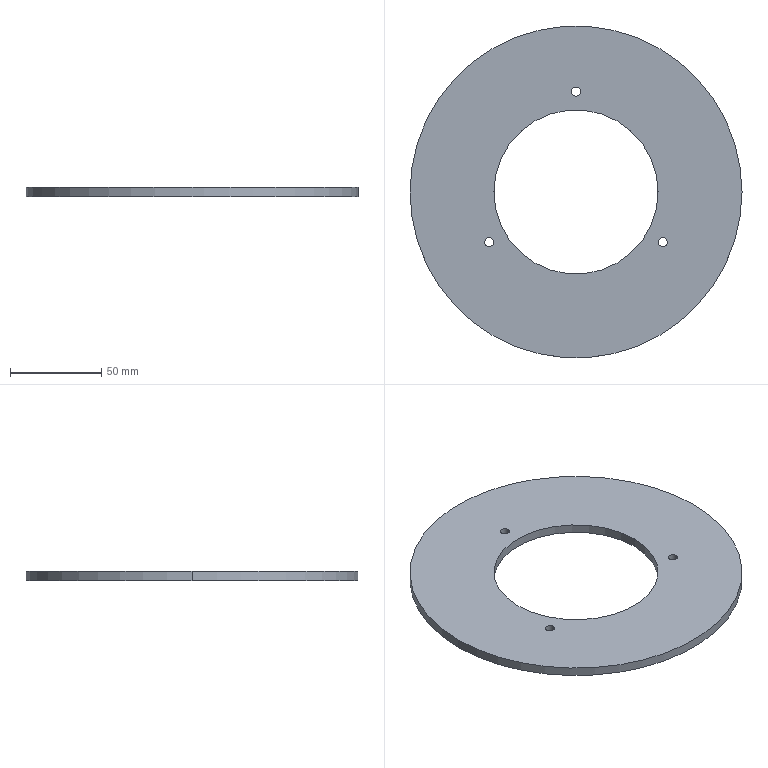Part | SolidWorks | features Extrusion 1 | 1 solid | 12 faces | box 182 x 182 x 5 mm | volume 97974 mm3 | cylinder 10 | plane 2 | commonest cylinder face diameters 5 x6 90 x2 182 x2
STEP:
#1=CARTESIAN_POINT('',(-50.131,-27.5,5.));
#2=VERTEX_POINT('',#1);
#3=CARTESIAN_POINT('',(-45.131,-27.5,5.));
#4=VERTEX_POINT('',#3);
#5=CARTESIAN_POINT('',(-47.631,-27.5,5.));
#6=DIRECTION('',(0.,0.,1.));
#7=DIRECTION('',(1.,0.,0.));
#8=AXIS2_PLACEMENT_3D('',#5,#6,#7);
#9=CIRCLE('',#8,2.5);
#10=EDGE_CURVE('',#2,#4,#9,.T.);
#11=ORIENTED_EDGE('',*,*,#10,.T.);
#12=CARTESIAN_POINT('',(-45.131,-27.5,0.));
#13=VERTEX_POINT('',#12);
#14=CARTESIAN_POINT('',(-45.131,-27.5,5.));
#15=DIRECTION('',(0.,0.,-1.));
#16=VECTOR('',#15,1000.);
#17=LINE('',#14,#16);
#18=EDGE_CURVE('',#4,#13,#17,.T.);
#19=ORIENTED_EDGE('',*,*,#18,.T.);
#20=CARTESIAN_POINT('',(-50.131,-27.5,0.));
#21=VERTEX_POINT('',#20);
#22=CARTESIAN_POINT('',(-47.631,-27.5,0.));
#23=DIRECTION('',(0.,0.,1.));
#24=DIRECTION('',(1.,0.,0.));
#25=AXIS2_PLACEMENT_3D('',#22,#23,#24);
#26=CIRCLE('',#25,2.5);
#27=EDGE_CURVE('',#21,#13,#26,.T.);
#28=ORIENTED_EDGE('',*,*,#27,.F.);
#29=CARTESIAN_POINT('',(-50.131,-27.5,5.));
#30=DIRECTION('',(0.,0.,-1.));
#31=VECTOR('',#30,1000.);
#32=LINE('',#29,#31);
#33=EDGE_CURVE('',#2,#21,#32,.T.);
#34=ORIENTED_EDGE('',*,*,#33,.F.);
#35=EDGE_LOOP('',(#11,#19,#28,#34));
#36=FACE_OUTER_BOUND('',#35,.T.);
#37=CARTESIAN_POINT('',(-47.631,-27.5,5.));
#38=DIRECTION('',(0.,0.,-1.));
#39=DIRECTION('',(-1.,0.,0.));
#40=AXIS2_PLACEMENT_3D('',#37,#38,#39);
#41=CYLINDRICAL_SURFACE('',#40,2.5);
#42=ADVANCED_FACE('',(#36),#41,.F.);
#43=CARTESIAN_POINT('',(45.131,-27.5,5.));
#44=VERTEX_POINT('',#43);
#45=CARTESIAN_POINT('',(50.131,-27.5,5.));
#46=VERTEX_POINT('',#45);
#47=CARTESIAN_POINT('',(47.631,-27.5,5.));
#48=DIRECTION('',(0.,0.,1.));
#49=DIRECTION('',(1.,0.,0.));
#50=AXIS2_PLACEMENT_3D('',#47,#48,#49);
#51=CIRCLE('',#50,2.5);
#52=EDGE_CURVE('',#44,#46,#51,.T.);
#53=ORIENTED_EDGE('',*,*,#52,.T.);
#54=CARTESIAN_POINT('',(50.131,-27.5,0.));
#55=VERTEX_POINT('',#54);
#56=CARTESIAN_POINT('',(50.131,-27.5,5.));
#57=DIRECTION('',(0.,0.,-1.));
#58=VECTOR('',#57,1000.);
#59=LINE('',#56,#58);
#60=EDGE_CURVE('',#46,#55,#59,.T.);
#61=ORIENTED_EDGE('',*,*,#60,.T.);
#62=CARTESIAN_POINT('',(45.131,-27.5,0.));
#63=VERTEX_POINT('',#62);
#64=CARTESIAN_POINT('',(47.631,-27.5,0.));
#65=DIRECTION('',(0.,0.,1.));
#66=DIRECTION('',(1.,0.,0.));
#67=AXIS2_PLACEMENT_3D('',#64,#65,#66);
#68=CIRCLE('',#67,2.5);
#69=EDGE_CURVE('',#63,#55,#68,.T.);
#70=ORIENTED_EDGE('',*,*,#69,.F.);
#71=CARTESIAN_POINT('',(45.131,-27.5,5.));
#72=DIRECTION('',(0.,0.,-1.));
#73=VECTOR('',#72,1000.);
#74=LINE('',#71,#73);
#75=EDGE_CURVE('',#44,#63,#74,.T.);
#76=ORIENTED_EDGE('',*,*,#75,.F.);
#77=EDGE_LOOP('',(#53,#61,#70,#76));
#78=FACE_OUTER_BOUND('',#77,.T.);
#79=CARTESIAN_POINT('',(47.631,-27.5,5.));
#80=DIRECTION('',(0.,0.,-1.));
#81=DIRECTION('',(-1.,0.,0.));
#82=AXIS2_PLACEMENT_3D('',#79,#80,#81);
#83=CYLINDRICAL_SURFACE('',#82,2.5);
#84=ADVANCED_FACE('',(#78),#83,.F.);
#85=CARTESIAN_POINT('',(-2.5,55.,5.));
#86=VERTEX_POINT('',#85);
#87=CARTESIAN_POINT('',(2.5,55.,5.));
#88=VERTEX_POINT('',#87);
#89=CARTESIAN_POINT('',(0.,55.,5.));
#90=DIRECTION('',(0.,0.,1.));
#91=DIRECTION('',(1.,0.,0.));
#92=AXIS2_PLACEMENT_3D('',#89,#90,#91);
#93=CIRCLE('',#92,2.5);
#94=EDGE_CURVE('',#86,#88,#93,.T.);
#95=ORIENTED_EDGE('',*,*,#94,.T.);
#96=CARTESIAN_POINT('',(2.5,55.,0.));
#97=VERTEX_POINT('',#96);
#98=CARTESIAN_POINT('',(2.5,55.,5.));
#99=DIRECTION('',(0.,0.,-1.));
#100=VECTOR('',#99,1000.);
#101=LINE('',#98,#100);
#102=EDGE_CURVE('',#88,#97,#101,.T.);
#103=ORIENTED_EDGE('',*,*,#102,.T.);
#104=CARTESIAN_POINT('',(-2.5,55.,0.));
#105=VERTEX_POINT('',#104);
#106=CARTESIAN_POINT('',(0.,55.,0.));
#107=DIRECTION('',(0.,0.,1.));
#108=DIRECTION('',(1.,0.,0.));
#109=AXIS2_PLACEMENT_3D('',#106,#107,#108);
#110=CIRCLE('',#109,2.5);
#111=EDGE_CURVE('',#105,#97,#110,.T.);
#112=ORIENTED_EDGE('',*,*,#111,.F.);
#113=CARTESIAN_POINT('',(-2.5,55.,5.));
#114=DIRECTION('',(0.,0.,-1.));
#115=VECTOR('',#114,1000.);
#116=LINE('',#113,#115);
#117=EDGE_CURVE('',#86,#105,#116,.T.);
#118=ORIENTED_EDGE('',*,*,#117,.F.);
#119=EDGE_LOOP('',(#95,#103,#112,#118));
#120=FACE_OUTER_BOUND('',#119,.T.);
#121=CARTESIAN_POINT('',(0.,55.,5.));
#122=DIRECTION('',(0.,0.,-1.));
#123=DIRECTION('',(-1.,0.,0.));
#124=AXIS2_PLACEMENT_3D('',#121,#122,#123);
#125=CYLINDRICAL_SURFACE('',#124,2.5);
#126=ADVANCED_FACE('',(#120),#125,.F.);
#127=CARTESIAN_POINT('',(-45.,0.,5.));
#128=VERTEX_POINT('',#127);
#129=CARTESIAN_POINT('',(45.,0.,5.));
#130=VERTEX_POINT('',#129);
#131=CARTESIAN_POINT('',(0.,0.,5.));
#132=DIRECTION('',(0.,0.,1.));
#133=DIRECTION('',(1.,0.,0.));
#134=AXIS2_PLACEMENT_3D('',#131,#132,#133);
#135=CIRCLE('',#134,45.);
#136=EDGE_CURVE('',#128,#130,#135,.T.);
#137=ORIENTED_EDGE('',*,*,#136,.T.);
#138=CARTESIAN_POINT('',(45.,0.,0.));
#139=VERTEX_POINT('',#138);
#140=CARTESIAN_POINT('',(45.,0.,5.));
#141=DIRECTION('',(0.,0.,-1.));
#142=VECTOR('',#141,1000.);
#143=LINE('',#140,#142);
#144=EDGE_CURVE('',#130,#139,#143,.T.);
#145=ORIENTED_EDGE('',*,*,#144,.T.);
#146=CARTESIAN_POINT('',(-45.,0.,0.));
#147=VERTEX_POINT('',#146);
#148=CARTESIAN_POINT('',(0.,0.,0.));
#149=DIRECTION('',(0.,0.,1.));
#150=DIRECTION('',(1.,0.,0.));
#151=AXIS2_PLACEMENT_3D('',#148,#149,#150);
#152=CIRCLE('',#151,45.);
#153=EDGE_CURVE('',#147,#139,#152,.T.);
#154=ORIENTED_EDGE('',*,*,#153,.F.);
#155=CARTESIAN_POINT('',(-45.,0.,5.));
#156=DIRECTION('',(0.,0.,-1.));
#157=VECTOR('',#156,1000.);
#158=LINE('',#155,#157);
#159=EDGE_CURVE('',#128,#147,#158,.T.);
#160=ORIENTED_EDGE('',*,*,#159,.F.);
#161=EDGE_LOOP('',(#137,#145,#154,#160));
#162=FACE_OUTER_BOUND('',#161,.T.);
#163=CARTESIAN_POINT('',(0.,0.,5.));
#164=DIRECTION('',(0.,0.,-1.));
#165=DIRECTION('',(-1.,0.,0.));
#166=AXIS2_PLACEMENT_3D('',#163,#164,#165);
#167=CYLINDRICAL_SURFACE('',#166,45.);
#168=ADVANCED_FACE('',(#162),#167,.F.);
#169=CARTESIAN_POINT('',(91.,0.,5.));
#170=VERTEX_POINT('',#169);
#171=CARTESIAN_POINT('',(-91.,0.,5.));
#172=VERTEX_POINT('',#171);
#173=CARTESIAN_POINT('',(0.,0.,5.));
#174=DIRECTION('',(0.,0.,1.));
#175=DIRECTION('',(1.,0.,0.));
#176=AXIS2_PLACEMENT_3D('',#173,#174,#175);
#177=CIRCLE('',#176,91.);
#178=EDGE_CURVE('',#170,#172,#177,.T.);
#179=ORIENTED_EDGE('',*,*,#178,.F.);
#180=CARTESIAN_POINT('',(91.,0.,0.));
#181=VERTEX_POINT('',#180);
#182=CARTESIAN_POINT('',(91.,0.,5.));
#183=DIRECTION('',(0.,0.,-1.));
#184=VECTOR('',#183,1000.);
#185=LINE('',#182,#184);
#186=EDGE_CURVE('',#170,#181,#185,.T.);
#187=ORIENTED_EDGE('',*,*,#186,.T.);
#188=CARTESIAN_POINT('',(-91.,0.,0.));
#189=VERTEX_POINT('',#188);
#190=CARTESIAN_POINT('',(0.,0.,0.));
#191=DIRECTION('',(0.,0.,1.));
#192=DIRECTION('',(1.,0.,0.));
#193=AXIS2_PLACEMENT_3D('',#190,#191,#192);
#194=CIRCLE('',#193,91.);
#195=EDGE_CURVE('',#181,#189,#194,.T.);
#196=ORIENTED_EDGE('',*,*,#195,.T.);
#197=CARTESIAN_POINT('',(-91.,0.,5.));
#198=DIRECTION('',(0.,0.,-1.));
#199=VECTOR('',#198,1000.);
#200=LINE('',#197,#199);
#201=EDGE_CURVE('',#172,#189,#200,.T.);
#202=ORIENTED_EDGE('',*,*,#201,.F.);
#203=EDGE_LOOP('',(#179,#187,#196,#202));
#204=FACE_OUTER_BOUND('',#203,.T.);
#205=CARTESIAN_POINT('',(0.,0.,5.));
#206=DIRECTION('',(0.,0.,-1.));
#207=DIRECTION('',(-1.,0.,0.));
#208=AXIS2_PLACEMENT_3D('',#205,#206,#207);
#209=CYLINDRICAL_SURFACE('',#208,91.);
#210=ADVANCED_FACE('',(#204),#209,.T.);
#211=ORIENTED_EDGE('',*,*,#52,.F.);
#212=CARTESIAN_POINT('',(47.631,-27.5,5.));
#213=DIRECTION('',(0.,0.,1.));
#214=DIRECTION('',(1.,0.,0.));
#215=AXIS2_PLACEMENT_3D('',#212,#213,#214);
#216=CIRCLE('',#215,2.5);
#217=EDGE_CURVE('',#46,#44,#216,.T.);
#218=ORIENTED_EDGE('',*,*,#217,.F.);
#219=EDGE_LOOP('',(#211,#218));
#220=FACE_BOUND('',#219,.T.);
#221=ORIENTED_EDGE('',*,*,#136,.F.);
#222=CARTESIAN_POINT('',(0.,0.,5.));
#223=DIRECTION('',(0.,0.,1.));
#224=DIRECTION('',(1.,0.,0.));
#225=AXIS2_PLACEMENT_3D('',#222,#223,#224);
#226=CIRCLE('',#225,45.);
#227=EDGE_CURVE('',#130,#128,#226,.T.);
#228=ORIENTED_EDGE('',*,*,#227,.F.);
#229=EDGE_LOOP('',(#221,#228));
#230=FACE_BOUND('',#229,.T.);
#231=CARTESIAN_POINT('',(0.,0.,5.));
#232=DIRECTION('',(0.,0.,1.));
#233=DIRECTION('',(1.,0.,0.));
#234=AXIS2_PLACEMENT_3D('',#231,#232,#233);
#235=CIRCLE('',#234,91.);
#236=EDGE_CURVE('',#172,#170,#235,.T.);
#237=ORIENTED_EDGE('',*,*,#236,.T.);
#238=ORIENTED_EDGE('',*,*,#178,.T.);
#239=EDGE_LOOP('',(#237,#238));
#240=FACE_OUTER_BOUND('',#239,.T.);
#241=ORIENTED_EDGE('',*,*,#94,.F.);
#242=CARTESIAN_POINT('',(0.,55.,5.));
#243=DIRECTION('',(0.,0.,1.));
#244=DIRECTION('',(1.,0.,0.));
#245=AXIS2_PLACEMENT_3D('',#242,#243,#244);
#246=CIRCLE('',#245,2.5);
#247=EDGE_CURVE('',#88,#86,#246,.T.);
#248=ORIENTED_EDGE('',*,*,#247,.F.);
#249=EDGE_LOOP('',(#241,#248));
#250=FACE_BOUND('',#249,.T.);
#251=ORIENTED_EDGE('',*,*,#10,.F.);
#252=CARTESIAN_POINT('',(-47.631,-27.5,5.));
#253=DIRECTION('',(0.,0.,1.));
#254=DIRECTION('',(1.,0.,0.));
#255=AXIS2_PLACEMENT_3D('',#252,#253,#254);
#256=CIRCLE('',#255,2.5);
#257=EDGE_CURVE('',#4,#2,#256,.T.);
#258=ORIENTED_EDGE('',*,*,#257,.F.);
#259=EDGE_LOOP('',(#251,#258));
#260=FACE_BOUND('',#259,.T.);
#261=CARTESIAN_POINT('',(0.,0.,5.));
#262=DIRECTION('',(0.,0.,1.));
#263=DIRECTION('',(1.,0.,0.));
#264=AXIS2_PLACEMENT_3D('',#261,#262,#263);
#265=PLANE('',#264);
#266=ADVANCED_FACE('',(#220,#230,#240,#250,#260),#265,.T.);
#267=CARTESIAN_POINT('',(0.,0.,0.));
#268=DIRECTION('',(0.,0.,1.));
#269=DIRECTION('',(1.,0.,0.));
#270=AXIS2_PLACEMENT_3D('',#267,#268,#269);
#271=CIRCLE('',#270,91.);
#272=EDGE_CURVE('',#189,#181,#271,.T.);
#273=ORIENTED_EDGE('',*,*,#272,.F.);
#274=ORIENTED_EDGE('',*,*,#195,.F.);
#275=EDGE_LOOP('',(#273,#274));
#276=FACE_OUTER_BOUND('',#275,.T.);
#277=ORIENTED_EDGE('',*,*,#153,.T.);
#278=CARTESIAN_POINT('',(0.,0.,0.));
#279=DIRECTION('',(0.,0.,1.));
#280=DIRECTION('',(1.,0.,0.));
#281=AXIS2_PLACEMENT_3D('',#278,#279,#280);
#282=CIRCLE('',#281,45.);
#283=EDGE_CURVE('',#139,#147,#282,.T.);
#284=ORIENTED_EDGE('',*,*,#283,.T.);
#285=EDGE_LOOP('',(#277,#284));
#286=FACE_BOUND('',#285,.T.);
#287=ORIENTED_EDGE('',*,*,#111,.T.);
#288=CARTESIAN_POINT('',(0.,55.,0.));
#289=DIRECTION('',(0.,0.,1.));
#290=DIRECTION('',(1.,0.,0.));
#291=AXIS2_PLACEMENT_3D('',#288,#289,#290);
#292=CIRCLE('',#291,2.5);
#293=EDGE_CURVE('',#97,#105,#292,.T.);
#294=ORIENTED_EDGE('',*,*,#293,.T.);
#295=EDGE_LOOP('',(#287,#294));
#296=FACE_BOUND('',#295,.T.);
#297=ORIENTED_EDGE('',*,*,#69,.T.);
#298=CARTESIAN_POINT('',(47.631,-27.5,0.));
#299=DIRECTION('',(0.,0.,1.));
#300=DIRECTION('',(1.,0.,0.));
#301=AXIS2_PLACEMENT_3D('',#298,#299,#300);
#302=CIRCLE('',#301,2.5);
#303=EDGE_CURVE('',#55,#63,#302,.T.);
#304=ORIENTED_EDGE('',*,*,#303,.T.);
#305=EDGE_LOOP('',(#297,#304));
#306=FACE_BOUND('',#305,.T.);
#307=ORIENTED_EDGE('',*,*,#27,.T.);
#308=CARTESIAN_POINT('',(-47.631,-27.5,0.));
#309=DIRECTION('',(0.,0.,1.));
#310=DIRECTION('',(1.,0.,0.));
#311=AXIS2_PLACEMENT_3D('',#308,#309,#310);
#312=CIRCLE('',#311,2.5);
#313=EDGE_CURVE('',#13,#21,#312,.T.);
#314=ORIENTED_EDGE('',*,*,#313,.T.);
#315=EDGE_LOOP('',(#307,#314));
#316=FACE_BOUND('',#315,.T.);
#317=CARTESIAN_POINT('',(0.,0.,0.));
#318=DIRECTION('',(0.,0.,1.));
#319=DIRECTION('',(1.,0.,0.));
#320=AXIS2_PLACEMENT_3D('',#317,#318,#319);
#321=PLANE('',#320);
#322=ADVANCED_FACE('',(#276,#286,#296,#306,#316),#321,.F.);
#323=ORIENTED_EDGE('',*,*,#186,.F.);
#324=ORIENTED_EDGE('',*,*,#236,.F.);
#325=ORIENTED_EDGE('',*,*,#201,.T.);
#326=ORIENTED_EDGE('',*,*,#272,.T.);
#327=EDGE_LOOP('',(#323,#324,#325,#326));
#328=FACE_OUTER_BOUND('',#327,.T.);
#329=CARTESIAN_POINT('',(0.,0.,5.));
#330=DIRECTION('',(0.,0.,-1.));
#331=DIRECTION('',(-1.,0.,0.));
#332=AXIS2_PLACEMENT_3D('',#329,#330,#331);
#333=CYLINDRICAL_SURFACE('',#332,91.);
#334=ADVANCED_FACE('',(#328),#333,.T.);
#335=ORIENTED_EDGE('',*,*,#144,.F.);
#336=ORIENTED_EDGE('',*,*,#227,.T.);
#337=ORIENTED_EDGE('',*,*,#159,.T.);
#338=ORIENTED_EDGE('',*,*,#283,.F.);
#339=EDGE_LOOP('',(#335,#336,#337,#338));
#340=FACE_OUTER_BOUND('',#339,.T.);
#341=CARTESIAN_POINT('',(0.,0.,5.));
#342=DIRECTION('',(0.,0.,-1.));
#343=DIRECTION('',(-1.,0.,0.));
#344=AXIS2_PLACEMENT_3D('',#341,#342,#343);
#345=CYLINDRICAL_SURFACE('',#344,45.);
#346=ADVANCED_FACE('',(#340),#345,.F.);
#347=ORIENTED_EDGE('',*,*,#102,.F.);
#348=ORIENTED_EDGE('',*,*,#247,.T.);
#349=ORIENTED_EDGE('',*,*,#117,.T.);
#350=ORIENTED_EDGE('',*,*,#293,.F.);
#351=EDGE_LOOP('',(#347,#348,#349,#350));
#352=FACE_OUTER_BOUND('',#351,.T.);
#353=CARTESIAN_POINT('',(0.,55.,5.));
#354=DIRECTION('',(0.,0.,-1.));
#355=DIRECTION('',(-1.,0.,0.));
#356=AXIS2_PLACEMENT_3D('',#353,#354,#355);
#357=CYLINDRICAL_SURFACE('',#356,2.5);
#358=ADVANCED_FACE('',(#352),#357,.F.);
#359=ORIENTED_EDGE('',*,*,#60,.F.);
#360=ORIENTED_EDGE('',*,*,#217,.T.);
#361=ORIENTED_EDGE('',*,*,#75,.T.);
#362=ORIENTED_EDGE('',*,*,#303,.F.);
#363=EDGE_LOOP('',(#359,#360,#361,#362));
#364=FACE_OUTER_BOUND('',#363,.T.);
#365=CARTESIAN_POINT('',(47.631,-27.5,5.));
#366=DIRECTION('',(0.,0.,-1.));
#367=DIRECTION('',(-1.,0.,0.));
#368=AXIS2_PLACEMENT_3D('',#365,#366,#367);
#369=CYLINDRICAL_SURFACE('',#368,2.5);
#370=ADVANCED_FACE('',(#364),#369,.F.);
#371=ORIENTED_EDGE('',*,*,#18,.F.);
#372=ORIENTED_EDGE('',*,*,#257,.T.);
#373=ORIENTED_EDGE('',*,*,#33,.T.);
#374=ORIENTED_EDGE('',*,*,#313,.F.);
#375=EDGE_LOOP('',(#371,#372,#373,#374));
#376=FACE_OUTER_BOUND('',#375,.T.);
#377=CARTESIAN_POINT('',(-47.631,-27.5,5.));
#378=DIRECTION('',(0.,0.,-1.));
#379=DIRECTION('',(-1.,0.,0.));
#380=AXIS2_PLACEMENT_3D('',#377,#378,#379);
#381=CYLINDRICAL_SURFACE('',#380,2.5);
#382=ADVANCED_FACE('',(#376),#381,.F.);
#383=CLOSED_SHELL('',(#42,#84,#126,#168,#210,#266,#322,#334,#346,#358,#370,#382));
#384=MANIFOLD_SOLID_BREP('',#383);
#385=CARTESIAN_POINT('',(0.,0.,0.));
#386=DIRECTION('',(0.,0.,1.));
#387=DIRECTION('',(1.,0.,0.));
#388=AXIS2_PLACEMENT_3D('',#385,#386,#387);
#389=(LENGTH_UNIT()NAMED_UNIT(*)SI_UNIT(.MILLI.,.METRE.));
#390=UNCERTAINTY_MEASURE_WITH_UNIT(LENGTH_MEASURE(0.00001),#389,'','');
#391=(NAMED_UNIT(*)PLANE_ANGLE_UNIT()SI_UNIT($,.RADIAN.));
#392=(NAMED_UNIT(*)SI_UNIT($,.STERADIAN.)SOLID_ANGLE_UNIT());
#393=(GEOMETRIC_REPRESENTATION_CONTEXT(3)GLOBAL_UNCERTAINTY_ASSIGNED_CONTEXT((#390))GLOBAL_UNIT_ASSIGNED_CONTEXT((#389,#391,#392))REPRESENTATION_CONTEXT('',''));
#394=ADVANCED_BREP_SHAPE_REPRESENTATION('',(#384,#388),#393);